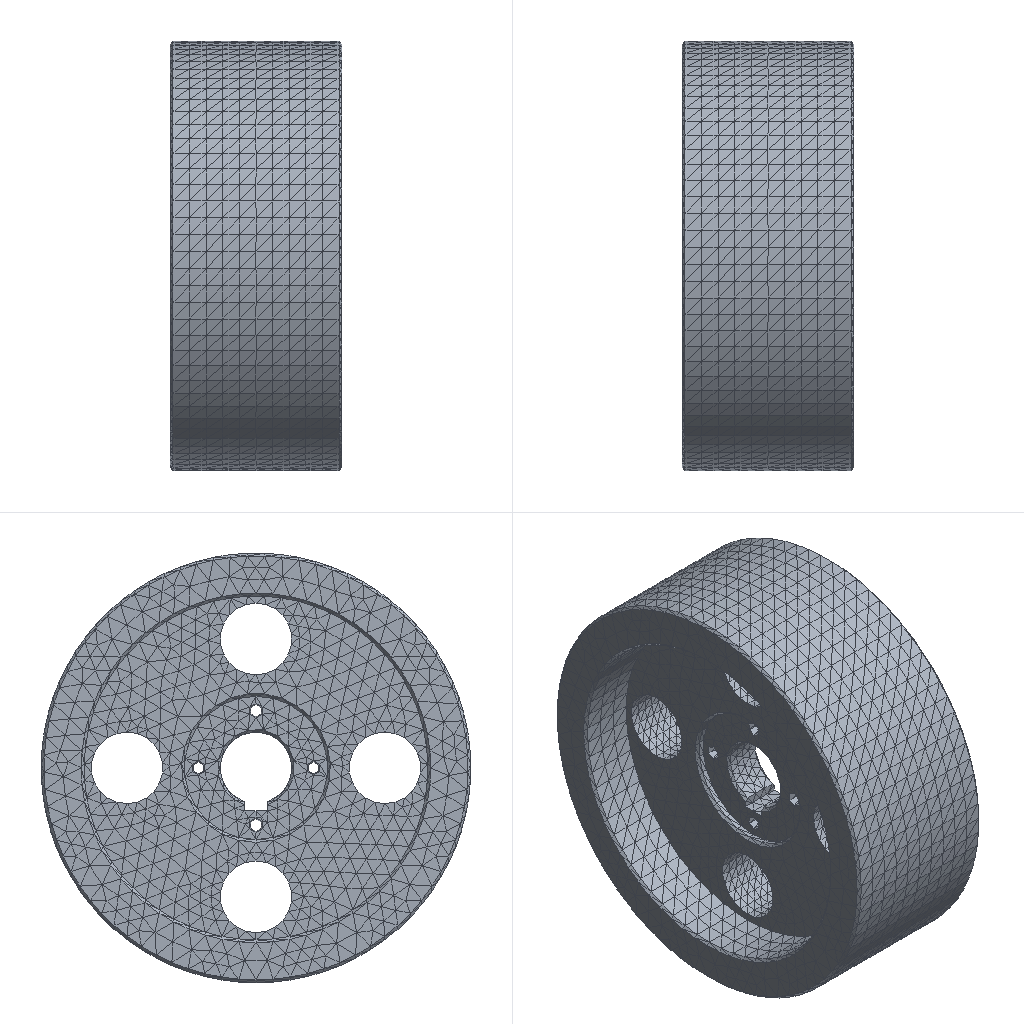Simulation study | nx simcenter
Set-up summary:
category,name,step,type,value,unit,region
solver,nx_nastran (Simcenter)
units,not stated in the deck,,not stated
analysis,deck,,static,static
analysis,solution,,SOL,101
load_step,SUBCASE 1,1,SUBCASE,SPC=1 LOAD=2
load_step,requested,,,1
mesh,nodes,,,27319
mesh,elements,,,15339
element_type,CTETRA,,solid,15339
load,nodal force total,,FX,0.0,model units
load,nodal force total,,FY,0.0,model units
load,nodal force total,,FZ,-5000000.07,model units
load,load commands in deck,,count,254
bc,support commands in deck,,count,3318
analysis,NX solution 0,,Structural,Linear Statics - Single Constraint
check,setup vs results,,match,every grid point's frame and coordinates and every element id; grid points of CTETRA elements
Nastran input file, long lists of numbers shortened:
$*$$$$$$$$$$$$$$$$$$$$$$$$$$$$$$$$$$$$$$$$$$$$$$$$$$$$$$$$$$$$$$$$$
$*
$*                    NX v10.0.0.24 TRANSLATOR
$*                    FOR NX NASTRAN VERSION 10.0
$ (33 more lines like these left out)
ASSIGN OUTPUT2='156_sim1-solution_1.op2' UNIT=12
$*
$*$$$$$$$$$$$$$$$$$$$$$$$$$$$$$$$$$$$
$*
$* EXECUTIVE CONTROL
$*
$*$$$$$$$$$$$$$$$$$$$$$$$$$$$$$$$$$$$
$*
ID,NASTRAN,156_sim1-solution_1
SOL 101
CEND
$*
$*$$$$$$$$$$$$$$$$$$$$$$$$$$$$$$$$$$$
$*
$* CASE CONTROL
$*
$*$$$$$$$$$$$$$$$$$$$$$$$$$$$$$$$$$$$
$*
TITLE = Solution 1
ECHO = NONE
SPC = 1
OUTPUT
BCRESULTS(TRACTION,FORCE,PLOT) = ALL
DISPLACEMENT(PLOT) = ALL
ESE(PLOT) = ALL
FORCE(PLOT,CORNER) = ALL
OLOAD(PLOT) = ALL
SPCFORCES(PLOT) = ALL
STRAIN(PLOT,FIBER,CORNER) = ALL
STRESS(PLOT,CORNER) = ALL
$*  NX Step: Subcase - Static Loads 1
SUBCASE 1
LABEL = Subcase - Static Loads 1
LOAD = 2
$*
$*$$$$$$$$$$$$$$$$$$$$$$$$$$$$$$$$$$$
$*
$* BULK DATA
$*
$*$$$$$$$$$$$$$$$$$$$$$$$$$$$$$$$$$$$
$*
BEGIN BULK
$*
$* PARAM CARDS
$*
PARAM      K6ROT100.0000
PARAM     OIBULK     YES
PARAM    OMACHPR     YES
PARAM       POST      -2
PARAM    POSTEXT     YES
PARAM    UNITSYS   MN-MM
$*
$* GRID CARDS
$*
GRID*              27276               0-3.000000000E+010.0000000000E+00+
*       -6.100000000E+01               0
GRID*              27277               0-3.000000000E+010.0000000000E+00+
*       -7.400000000E+01               0
$ (54634 more lines like these left out)
$*
$* ELEMENT CARDS
$*
$*  NX Mesh Collector: Solid(1)
$*  NX Mesh: 3d_mesh(1)
CTETRA         1       1   24836   17713   24835       1     951     952+
+          24851     953     954     955
CTETRA         2       1   15312   19397   26532   26285     956     957+
+          15441     958   22318   16011
$ (30674 more lines like these left out)
$*
$* PROPERTY CARDS
$*
$*  NX Property: PSOLID1
PSOLID         1       1       0                           SMECH
$*
$* MATERIAL CARDS
$*
$*  NX Material: 40Cr
MAT1           12.0600+8        0.3000007.8500-61.2000-5
$*
$* LOAD AND CONSTRAINT CARDS
$*
$*  NX Load and Constraint: Fixed(1)
SPC            1   19376  123456  0.0000
SPC            1   19377  123456  0.0000
SPC            1   19378  123456  0.0000
SPC            1   19379  123456  0.0000
$ (3314 more lines like these left out)
$*  NX Load and Constraint: Force(1)
FORCE          2   14871       021654.66  0.0000  0.0000-1.00000
FORCE          2   14872       021060.67  0.0000  0.0000-1.00000
FORCE          2   14873       022101.28  0.0000  0.0000-1.00000
FORCE          2   14874       027783.36  0.0000  0.0000-1.00000
$ (250 more lines like these left out)
ENDDATA cf0782fc
Results summary:
result,analysis,,,static
result,last_loadstep,,,1
result,primary field,,,displacements
result,max displacement,,,0.000968,model units
result,reaction total,,FX,0.1054,model units
result,reaction total,,FY,-0.03787,model units
result,reaction total,,FZ,5000010.0,model units
result,NX solution 0,,loadcases,1,mm